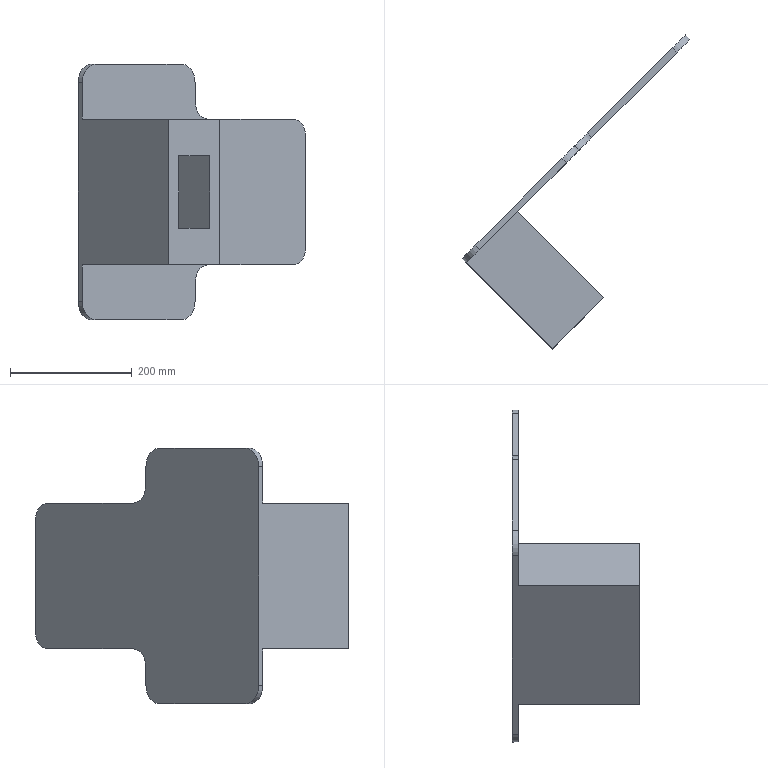Part | SolidWorks | 1 solid | 27 faces | box 374.767 x 516.188 x 420 mm | volume 5744112 mm3 | plane 19 | cylinder 8 | commonest cylinder face diameters 60 x8
STEP:
#1=CARTESIAN_POINT('',(-9.899,343.654,-1049.42));
#2=VERTEX_POINT('',#1);
#3=CARTESIAN_POINT('',(-60.811,292.742,-1049.42));
#4=VERTEX_POINT('',#3);
#5=CARTESIAN_POINT('',(-9.899,343.654,-1049.42));
#6=DIRECTION('',(-0.7071,-0.7071,0.));
#7=VECTOR('',#6,1000.);
#8=LINE('',#5,#7);
#9=EDGE_CURVE('',#2,#4,#8,.T.);
#10=ORIENTED_EDGE('',*,*,#9,.T.);
#11=CARTESIAN_POINT('',(-60.811,292.742,-1169.42));
#12=VERTEX_POINT('',#11);
#13=CARTESIAN_POINT('',(-60.811,292.742,-1169.42));
#14=DIRECTION('',(0.,0.,1.));
#15=VECTOR('',#14,1000.);
#16=LINE('',#13,#15);
#17=EDGE_CURVE('',#12,#4,#16,.T.);
#18=ORIENTED_EDGE('',*,*,#17,.F.);
#19=CARTESIAN_POINT('',(-9.899,343.654,-1169.42));
#20=VERTEX_POINT('',#19);
#21=CARTESIAN_POINT('',(-60.811,292.742,-1169.42));
#22=DIRECTION('',(0.7071,0.7071,0.));
#23=VECTOR('',#22,1000.);
#24=LINE('',#21,#23);
#25=EDGE_CURVE('',#12,#20,#24,.T.);
#26=ORIENTED_EDGE('',*,*,#25,.T.);
#27=CARTESIAN_POINT('',(-9.899,343.654,-1049.42));
#28=DIRECTION('',(0.,0.,-1.));
#29=VECTOR('',#28,1000.);
#30=LINE('',#27,#29);
#31=EDGE_CURVE('',#2,#20,#30,.T.);
#32=ORIENTED_EDGE('',*,*,#31,.F.);
#33=EDGE_LOOP('',(#10,#18,#26,#32));
#34=FACE_OUTER_BOUND('',#33,.T.);
#35=CARTESIAN_POINT('',(-77.782,275.772,-989.42));
#36=DIRECTION('',(0.7071,-0.7071,0.));
#37=DIRECTION('',(0.,0.,-1.));
#38=AXIS2_PLACEMENT_3D('',#35,#36,#37);
#39=PLANE('',#38);
#40=ADVANCED_FACE('',(#34),#39,.T.);
#41=CARTESIAN_POINT('',(131.522,202.233,-1169.42));
#42=VERTEX_POINT('',#41);
#43=CARTESIAN_POINT('',(80.61,151.321,-1169.42));
#44=VERTEX_POINT('',#43);
#45=CARTESIAN_POINT('',(131.522,202.233,-1169.42));
#46=DIRECTION('',(-0.7071,-0.7071,0.));
#47=VECTOR('',#46,1000.);
#48=LINE('',#45,#47);
#49=EDGE_CURVE('',#42,#44,#48,.T.);
#50=ORIENTED_EDGE('',*,*,#49,.F.);
#51=CARTESIAN_POINT('',(-9.899,343.654,-1169.42));
#52=DIRECTION('',(0.7071,-0.7071,0.));
#53=VECTOR('',#52,1000.);
#54=LINE('',#51,#53);
#55=EDGE_CURVE('',#20,#42,#54,.T.);
#56=ORIENTED_EDGE('',*,*,#55,.F.);
#57=ORIENTED_EDGE('',*,*,#25,.F.);
#58=CARTESIAN_POINT('',(80.61,151.321,-1169.42));
#59=DIRECTION('',(-0.7071,0.7071,0.));
#60=VECTOR('',#59,1000.);
#61=LINE('',#58,#60);
#62=EDGE_CURVE('',#44,#12,#61,.T.);
#63=ORIENTED_EDGE('',*,*,#62,.F.);
#64=EDGE_LOOP('',(#50,#56,#57,#63));
#65=FACE_OUTER_BOUND('',#64,.T.);
#66=CARTESIAN_POINT('',(80.61,151.321,-1169.42));
#67=DIRECTION('',(0.,0.,1.));
#68=DIRECTION('',(1.,0.,0.));
#69=AXIS2_PLACEMENT_3D('',#66,#67,#68);
#70=PLANE('',#69);
#71=ADVANCED_FACE('',(#65),#70,.T.);
#72=CARTESIAN_POINT('',(131.522,202.233,-1049.42));
#73=VERTEX_POINT('',#72);
#74=CARTESIAN_POINT('',(131.522,202.233,-1049.42));
#75=DIRECTION('',(0.,0.,-1.));
#76=VECTOR('',#75,1000.);
#77=LINE('',#74,#76);
#78=EDGE_CURVE('',#73,#42,#77,.T.);
#79=ORIENTED_EDGE('',*,*,#78,.F.);
#80=CARTESIAN_POINT('',(131.522,202.233,-1049.42));
#81=DIRECTION('',(-0.7071,0.7071,0.));
#82=VECTOR('',#81,1000.);
#83=LINE('',#80,#82);
#84=EDGE_CURVE('',#73,#2,#83,.T.);
#85=ORIENTED_EDGE('',*,*,#84,.T.);
#86=ORIENTED_EDGE('',*,*,#31,.T.);
#87=ORIENTED_EDGE('',*,*,#55,.T.);
#88=EDGE_LOOP('',(#79,#85,#86,#87));
#89=FACE_OUTER_BOUND('',#88,.T.);
#90=CARTESIAN_POINT('',(131.522,202.233,-1169.42));
#91=DIRECTION('',(-0.7071,-0.7071,0.));
#92=DIRECTION('',(-0.7071,0.7071,0.));
#93=AXIS2_PLACEMENT_3D('',#90,#91,#92);
#94=PLANE('',#93);
#95=ADVANCED_FACE('',(#89),#94,.T.);
#96=CARTESIAN_POINT('',(80.61,151.321,-1049.42));
#97=VERTEX_POINT('',#96);
#98=CARTESIAN_POINT('',(80.61,151.321,-1049.42));
#99=DIRECTION('',(0.7071,0.7071,0.));
#100=VECTOR('',#99,1000.);
#101=LINE('',#98,#100);
#102=EDGE_CURVE('',#97,#73,#101,.T.);
#103=ORIENTED_EDGE('',*,*,#102,.F.);
#104=CARTESIAN_POINT('',(-60.811,292.742,-1049.42));
#105=DIRECTION('',(0.7071,-0.7071,0.));
#106=VECTOR('',#105,1000.);
#107=LINE('',#104,#106);
#108=EDGE_CURVE('',#4,#97,#107,.T.);
#109=ORIENTED_EDGE('',*,*,#108,.F.);
#110=ORIENTED_EDGE('',*,*,#9,.F.);
#111=ORIENTED_EDGE('',*,*,#84,.F.);
#112=EDGE_LOOP('',(#103,#109,#110,#111));
#113=FACE_OUTER_BOUND('',#112,.T.);
#114=CARTESIAN_POINT('',(131.522,202.233,-1049.42));
#115=DIRECTION('',(0.,0.,-1.));
#116=DIRECTION('',(0.,-1.,0.));
#117=AXIS2_PLACEMENT_3D('',#114,#115,#116);
#118=PLANE('',#117);
#119=ADVANCED_FACE('',(#113),#118,.T.);
#120=CARTESIAN_POINT('',(80.61,151.321,-1169.42));
#121=DIRECTION('',(0.,0.,1.));
#122=VECTOR('',#121,1000.);
#123=LINE('',#120,#122);
#124=EDGE_CURVE('',#44,#97,#123,.T.);
#125=ORIENTED_EDGE('',*,*,#124,.F.);
#126=ORIENTED_EDGE('',*,*,#62,.T.);
#127=ORIENTED_EDGE('',*,*,#17,.T.);
#128=ORIENTED_EDGE('',*,*,#108,.T.);
#129=EDGE_LOOP('',(#125,#126,#127,#128));
#130=FACE_OUTER_BOUND('',#129,.T.);
#131=CARTESIAN_POINT('',(80.61,151.321,-1049.42));
#132=DIRECTION('',(0.7071,0.7071,0.));
#133=DIRECTION('',(0.,0.,-1.));
#134=AXIS2_PLACEMENT_3D('',#131,#132,#133);
#135=PLANE('',#134);
#136=ADVANCED_FACE('',(#130),#135,.T.);
#137=CARTESIAN_POINT('',(63.64,134.35,-989.42));
#138=VERTEX_POINT('',#137);
#139=CARTESIAN_POINT('',(-77.782,275.772,-989.42));
#140=VERTEX_POINT('',#139);
#141=CARTESIAN_POINT('',(63.64,134.35,-989.42));
#142=DIRECTION('',(-0.7071,0.7071,0.));
#143=VECTOR('',#142,1000.);
#144=LINE('',#141,#143);
#145=EDGE_CURVE('',#138,#140,#144,.T.);
#146=ORIENTED_EDGE('',*,*,#145,.F.);
#147=CARTESIAN_POINT('',(148.492,219.203,-989.42));
#148=VERTEX_POINT('',#147);
#149=CARTESIAN_POINT('',(148.492,219.203,-989.42));
#150=DIRECTION('',(-0.7071,-0.7071,0.));
#151=VECTOR('',#150,1000.);
#152=LINE('',#149,#151);
#153=EDGE_CURVE('',#148,#138,#152,.T.);
#154=ORIENTED_EDGE('',*,*,#153,.F.);
#155=CARTESIAN_POINT('',(7.071,360.624,-989.42));
#156=VERTEX_POINT('',#155);
#157=CARTESIAN_POINT('',(7.071,360.624,-989.42));
#158=DIRECTION('',(0.7071,-0.7071,0.));
#159=VECTOR('',#158,1000.);
#160=LINE('',#157,#159);
#161=EDGE_CURVE('',#156,#148,#160,.T.);
#162=ORIENTED_EDGE('',*,*,#161,.F.);
#163=CARTESIAN_POINT('',(-77.782,275.772,-989.42));
#164=DIRECTION('',(0.7071,0.7071,0.));
#165=VECTOR('',#164,1000.);
#166=LINE('',#163,#165);
#167=EDGE_CURVE('',#140,#156,#166,.T.);
#168=ORIENTED_EDGE('',*,*,#167,.F.);
#169=EDGE_LOOP('',(#146,#154,#162,#168));
#170=FACE_OUTER_BOUND('',#169,.T.);
#171=CARTESIAN_POINT('',(63.64,134.35,-989.42));
#172=DIRECTION('',(0.,0.,1.));
#173=DIRECTION('',(1.,0.,0.));
#174=AXIS2_PLACEMENT_3D('',#171,#172,#173);
#175=PLANE('',#174);
#176=ADVANCED_FACE('',(#170),#175,.T.);
#177=CARTESIAN_POINT('',(289.914,643.467,-1199.42));
#178=VERTEX_POINT('',#177);
#179=CARTESIAN_POINT('',(289.914,643.467,-1019.42));
#180=VERTEX_POINT('',#179);
#181=CARTESIAN_POINT('',(289.914,643.467,-1229.42));
#182=DIRECTION('',(0.,0.,1.));
#183=VECTOR('',#182,1000.);
#184=LINE('',#181,#183);
#185=EDGE_CURVE('',#178,#180,#184,.T.);
#186=ORIENTED_EDGE('',*,*,#185,.F.);
#187=CARTESIAN_POINT('',(282.843,650.538,-1199.42));
#188=VERTEX_POINT('',#187);
#189=CARTESIAN_POINT('',(431.335,502.046,-1199.42));
#190=DIRECTION('',(-0.7071,0.7071,0.));
#191=VECTOR('',#190,1000.);
#192=LINE('',#189,#191);
#193=EDGE_CURVE('',#178,#188,#192,.T.);
#194=ORIENTED_EDGE('',*,*,#193,.T.);
#195=CARTESIAN_POINT('',(282.843,650.538,-1019.42));
#196=VERTEX_POINT('',#195);
#197=CARTESIAN_POINT('',(282.843,650.538,-989.42));
#198=DIRECTION('',(0.,0.,-1.));
#199=VECTOR('',#198,1000.);
#200=LINE('',#197,#199);
#201=EDGE_CURVE('',#196,#188,#200,.T.);
#202=ORIENTED_EDGE('',*,*,#201,.F.);
#203=CARTESIAN_POINT('',(431.335,502.046,-1019.42));
#204=DIRECTION('',(0.7071,-0.7071,0.));
#205=VECTOR('',#204,1000.);
#206=LINE('',#203,#205);
#207=EDGE_CURVE('',#196,#180,#206,.T.);
#208=ORIENTED_EDGE('',*,*,#207,.T.);
#209=EDGE_LOOP('',(#186,#194,#202,#208));
#210=FACE_OUTER_BOUND('',#209,.T.);
#211=CARTESIAN_POINT('',(431.335,502.046,-1099.061));
#212=DIRECTION('',(0.7071,0.7071,0.));
#213=DIRECTION('',(0.,0.,-1.));
#214=AXIS2_PLACEMENT_3D('',#211,#212,#213);
#215=PLANE('',#214);
#216=ADVANCED_FACE('',(#210),#215,.T.);
#217=CARTESIAN_POINT('',(268.701,622.254,-989.42));
#218=VERTEX_POINT('',#217);
#219=CARTESIAN_POINT('',(128.787,482.34,-989.42));
#220=VERTEX_POINT('',#219);
#221=CARTESIAN_POINT('',(289.914,643.467,-989.42));
#222=DIRECTION('',(-0.7071,-0.7071,0.));
#223=VECTOR('',#222,1000.);
#224=LINE('',#221,#223);
#225=EDGE_CURVE('',#218,#220,#224,.T.);
#226=ORIENTED_EDGE('',*,*,#225,.F.);
#227=CARTESIAN_POINT('',(261.63,629.325,-989.42));
#228=VERTEX_POINT('',#227);
#229=CARTESIAN_POINT('',(410.122,480.833,-989.42));
#230=DIRECTION('',(-0.7071,0.7071,0.));
#231=VECTOR('',#230,1000.);
#232=LINE('',#229,#231);
#233=EDGE_CURVE('',#218,#228,#232,.T.);
#234=ORIENTED_EDGE('',*,*,#233,.T.);
#235=CARTESIAN_POINT('',(121.716,489.411,-989.42));
#236=VERTEX_POINT('',#235);
#237=CARTESIAN_POINT('',(100.503,468.198,-989.42));
#238=DIRECTION('',(0.7071,0.7071,0.));
#239=VECTOR('',#238,1000.);
#240=LINE('',#237,#239);
#241=EDGE_CURVE('',#236,#228,#240,.T.);
#242=ORIENTED_EDGE('',*,*,#241,.F.);
#243=CARTESIAN_POINT('',(128.787,482.34,-989.42));
#244=DIRECTION('',(0.7071,-0.7071,0.));
#245=VECTOR('',#244,1000.);
#246=LINE('',#243,#245);
#247=EDGE_CURVE('',#236,#220,#246,.T.);
#248=ORIENTED_EDGE('',*,*,#247,.T.);
#249=EDGE_LOOP('',(#226,#234,#242,#248));
#250=FACE_OUTER_BOUND('',#249,.T.);
#251=CARTESIAN_POINT('',(63.64,134.35,-989.42));
#252=DIRECTION('',(0.,0.,1.));
#253=DIRECTION('',(1.,0.,0.));
#254=AXIS2_PLACEMENT_3D('',#251,#252,#253);
#255=PLANE('',#254);
#256=ADVANCED_FACE('',(#250),#255,.T.);
#257=CARTESIAN_POINT('',(107.574,461.127,-929.42));
#258=VERTEX_POINT('',#257);
#259=CARTESIAN_POINT('',(107.574,461.127,-959.42));
#260=VERTEX_POINT('',#259);
#261=CARTESIAN_POINT('',(107.574,461.127,-899.42));
#262=DIRECTION('',(0.,0.,-1.));
#263=VECTOR('',#262,1000.);
#264=LINE('',#261,#263);
#265=EDGE_CURVE('',#258,#260,#264,.T.);
#266=ORIENTED_EDGE('',*,*,#265,.T.);
#267=CARTESIAN_POINT('',(100.503,468.198,-959.42));
#268=VERTEX_POINT('',#267);
#269=CARTESIAN_POINT('',(100.503,468.198,-959.42));
#270=DIRECTION('',(-0.7071,0.7071,0.));
#271=VECTOR('',#270,1000.);
#272=LINE('',#269,#271);
#273=EDGE_CURVE('',#260,#268,#272,.T.);
#274=ORIENTED_EDGE('',*,*,#273,.T.);
#275=CARTESIAN_POINT('',(100.503,468.198,-929.42));
#276=VERTEX_POINT('',#275);
#277=CARTESIAN_POINT('',(100.503,468.198,-899.42));
#278=DIRECTION('',(0.,0.,-1.));
#279=VECTOR('',#278,1000.);
#280=LINE('',#277,#279);
#281=EDGE_CURVE('',#276,#268,#280,.T.);
#282=ORIENTED_EDGE('',*,*,#281,.F.);
#283=CARTESIAN_POINT('',(100.503,468.198,-929.42));
#284=DIRECTION('',(0.7071,-0.7071,0.));
#285=VECTOR('',#284,1000.);
#286=LINE('',#283,#285);
#287=EDGE_CURVE('',#276,#258,#286,.T.);
#288=ORIENTED_EDGE('',*,*,#287,.T.);
#289=EDGE_LOOP('',(#266,#274,#282,#288));
#290=FACE_OUTER_BOUND('',#289,.T.);
#291=CARTESIAN_POINT('',(100.503,468.198,-899.42));
#292=DIRECTION('',(0.7071,0.7071,0.));
#293=DIRECTION('',(0.,0.,-1.));
#294=AXIS2_PLACEMENT_3D('',#291,#292,#293);
#295=PLANE('',#294);
#296=ADVANCED_FACE('',(#290),#295,.T.);
#297=CARTESIAN_POINT('',(-63.64,304.056,-899.42));
#298=VERTEX_POINT('',#297);
#299=CARTESIAN_POINT('',(79.289,446.985,-899.42));
#300=VERTEX_POINT('',#299);
#301=CARTESIAN_POINT('',(-84.853,282.843,-899.42));
#302=DIRECTION('',(0.7071,0.7071,0.));
#303=VECTOR('',#302,1000.);
#304=LINE('',#301,#303);
#305=EDGE_CURVE('',#298,#300,#304,.T.);
#306=ORIENTED_EDGE('',*,*,#305,.F.);
#307=CARTESIAN_POINT('',(-56.569,296.985,-899.42));
#308=VERTEX_POINT('',#307);
#309=CARTESIAN_POINT('',(-63.64,304.056,-899.42));
#310=DIRECTION('',(0.7071,-0.7071,0.));
#311=VECTOR('',#310,1000.);
#312=LINE('',#309,#311);
#313=EDGE_CURVE('',#298,#308,#312,.T.);
#314=ORIENTED_EDGE('',*,*,#313,.T.);
#315=CARTESIAN_POINT('',(86.36,439.914,-899.42));
#316=VERTEX_POINT('',#315);
#317=CARTESIAN_POINT('',(-77.782,275.772,-899.42));
#318=DIRECTION('',(0.7071,0.7071,0.));
#319=VECTOR('',#318,1000.);
#320=LINE('',#317,#319);
#321=EDGE_CURVE('',#308,#316,#320,.T.);
#322=ORIENTED_EDGE('',*,*,#321,.T.);
#323=CARTESIAN_POINT('',(79.289,446.985,-899.42));
#324=DIRECTION('',(-0.7071,0.7071,0.));
#325=VECTOR('',#324,1000.);
#326=LINE('',#323,#325);
#327=EDGE_CURVE('',#316,#300,#326,.T.);
#328=ORIENTED_EDGE('',*,*,#327,.T.);
#329=EDGE_LOOP('',(#306,#314,#322,#328));
#330=FACE_OUTER_BOUND('',#329,.T.);
#331=CARTESIAN_POINT('',(-84.853,282.843,-899.42));
#332=DIRECTION('',(0.,0.,1.));
#333=DIRECTION('',(0.7071,0.7071,0.));
#334=AXIS2_PLACEMENT_3D('',#331,#332,#333);
#335=PLANE('',#334);
#336=ADVANCED_FACE('',(#330),#335,.T.);
#337=CARTESIAN_POINT('',(79.289,446.985,-1319.42));
#338=VERTEX_POINT('',#337);
#339=CARTESIAN_POINT('',(-63.64,304.056,-1319.42));
#340=VERTEX_POINT('',#339);
#341=CARTESIAN_POINT('',(100.503,468.198,-1319.42));
#342=DIRECTION('',(-0.7071,-0.7071,0.));
#343=VECTOR('',#342,1000.);
#344=LINE('',#341,#343);
#345=EDGE_CURVE('',#338,#340,#344,.T.);
#346=ORIENTED_EDGE('',*,*,#345,.F.);
#347=CARTESIAN_POINT('',(86.36,439.914,-1319.42));
#348=VERTEX_POINT('',#347);
#349=CARTESIAN_POINT('',(79.289,446.985,-1319.42));
#350=DIRECTION('',(0.7071,-0.7071,0.));
#351=VECTOR('',#350,1000.);
#352=LINE('',#349,#351);
#353=EDGE_CURVE('',#338,#348,#352,.T.);
#354=ORIENTED_EDGE('',*,*,#353,.T.);
#355=CARTESIAN_POINT('',(-56.569,296.985,-1319.42));
#356=VERTEX_POINT('',#355);
#357=CARTESIAN_POINT('',(107.574,461.127,-1319.42));
#358=DIRECTION('',(-0.7071,-0.7071,0.));
#359=VECTOR('',#358,1000.);
#360=LINE('',#357,#359);
#361=EDGE_CURVE('',#348,#356,#360,.T.);
#362=ORIENTED_EDGE('',*,*,#361,.T.);
#363=CARTESIAN_POINT('',(-63.64,304.056,-1319.42));
#364=DIRECTION('',(-0.7071,0.7071,0.));
#365=VECTOR('',#364,1000.);
#366=LINE('',#363,#365);
#367=EDGE_CURVE('',#356,#340,#366,.T.);
#368=ORIENTED_EDGE('',*,*,#367,.T.);
#369=EDGE_LOOP('',(#346,#354,#362,#368));
#370=FACE_OUTER_BOUND('',#369,.T.);
#371=CARTESIAN_POINT('',(100.503,468.198,-1319.42));
#372=DIRECTION('',(0.,0.,-1.));
#373=DIRECTION('',(-0.7071,-0.7071,0.));
#374=AXIS2_PLACEMENT_3D('',#371,#372,#373);
#375=PLANE('',#374);
#376=ADVANCED_FACE('',(#370),#375,.T.);
#377=CARTESIAN_POINT('',(148.492,219.203,-1229.42));
#378=VERTEX_POINT('',#377);
#379=CARTESIAN_POINT('',(7.071,360.624,-1229.42));
#380=VERTEX_POINT('',#379);
#381=CARTESIAN_POINT('',(148.492,219.203,-1229.42));
#382=DIRECTION('',(-0.7071,0.7071,0.));
#383=VECTOR('',#382,1000.);
#384=LINE('',#381,#383);
#385=EDGE_CURVE('',#378,#380,#384,.T.);
#386=ORIENTED_EDGE('',*,*,#385,.F.);
#387=CARTESIAN_POINT('',(63.64,134.35,-1229.42));
#388=VERTEX_POINT('',#387);
#389=CARTESIAN_POINT('',(63.64,134.35,-1229.42));
#390=DIRECTION('',(0.7071,0.7071,0.));
#391=VECTOR('',#390,1000.);
#392=LINE('',#389,#391);
#393=EDGE_CURVE('',#388,#378,#392,.T.);
#394=ORIENTED_EDGE('',*,*,#393,.F.);
#395=CARTESIAN_POINT('',(-77.782,275.772,-1229.42));
#396=VERTEX_POINT('',#395);
#397=CARTESIAN_POINT('',(-77.782,275.772,-1229.42));
#398=DIRECTION('',(0.7071,-0.7071,0.));
#399=VECTOR('',#398,1000.);
#400=LINE('',#397,#399);
#401=EDGE_CURVE('',#396,#388,#400,.T.);
#402=ORIENTED_EDGE('',*,*,#401,.F.);
#403=CARTESIAN_POINT('',(7.071,360.624,-1229.42));
#404=DIRECTION('',(-0.7071,-0.7071,0.));
#405=VECTOR('',#404,1000.);
#406=LINE('',#403,#405);
#407=EDGE_CURVE('',#380,#396,#406,.T.);
#408=ORIENTED_EDGE('',*,*,#407,.F.);
#409=EDGE_LOOP('',(#386,#394,#402,#408));
#410=FACE_OUTER_BOUND('',#409,.T.);
#411=CARTESIAN_POINT('',(148.492,219.203,-1229.42));
#412=DIRECTION('',(0.,0.,-1.));
#413=DIRECTION('',(0.,-1.,0.));
#414=AXIS2_PLACEMENT_3D('',#411,#412,#413);
#415=PLANE('',#414);
#416=ADVANCED_FACE('',(#410),#415,.T.);
#417=CARTESIAN_POINT('',(-77.782,275.772,-929.42));
#418=VERTEX_POINT('',#417);
#419=CARTESIAN_POINT('',(-77.782,275.772,-989.42));
#420=DIRECTION('',(0.,0.,1.));
#421=VECTOR('',#420,1000.);
#422=LINE('',#419,#421);
#423=EDGE_CURVE('',#140,#418,#422,.T.);
#424=ORIENTED_EDGE('',*,*,#423,.T.);
#425=CARTESIAN_POINT('',(-84.853,282.843,-929.42));
#426=VERTEX_POINT('',#425);
#427=CARTESIAN_POINT('',(63.64,134.35,-929.42));
#428=DIRECTION('',(-0.7071,0.7071,0.));
#429=VECTOR('',#428,1000.);
#430=LINE('',#427,#429);
#431=EDGE_CURVE('',#418,#426,#430,.T.);
#432=ORIENTED_EDGE('',*,*,#431,.T.);
#433=CARTESIAN_POINT('',(-84.853,282.843,-1289.42));
#434=VERTEX_POINT('',#433);
#435=CARTESIAN_POINT('',(-84.853,282.843,-1319.42));
#436=DIRECTION('',(0.,0.,1.));
#437=VECTOR('',#436,1000.);
#438=LINE('',#435,#437);
#439=EDGE_CURVE('',#434,#426,#438,.T.);
#440=ORIENTED_EDGE('',*,*,#439,.F.);
#441=CARTESIAN_POINT('',(-77.782,275.772,-1289.42));
#442=VERTEX_POINT('',#441);
#443=CARTESIAN_POINT('',(63.64,134.35,-1289.42));
#444=DIRECTION('',(0.7071,-0.7071,0.));
#445=VECTOR('',#444,1000.);
#446=LINE('',#443,#445);
#447=EDGE_CURVE('',#434,#442,#446,.T.);
#448=ORIENTED_EDGE('',*,*,#447,.T.);
#449=CARTESIAN_POINT('',(-77.782,275.772,-1319.42));
#450=DIRECTION('',(0.,0.,1.));
#451=VECTOR('',#450,1000.);
#452=LINE('',#449,#451);
#453=EDGE_CURVE('',#442,#396,#452,.T.);
#454=ORIENTED_EDGE('',*,*,#453,.T.);
#455=ORIENTED_EDGE('',*,*,#401,.T.);
#456=CARTESIAN_POINT('',(63.64,134.35,-989.42));
#457=DIRECTION('',(0.,0.,-1.));
#458=VECTOR('',#457,1000.);
#459=LINE('',#456,#458);
#460=EDGE_CURVE('',#138,#388,#459,.T.);
#461=ORIENTED_EDGE('',*,*,#460,.F.);
#462=ORIENTED_EDGE('',*,*,#145,.T.);
#463=EDGE_LOOP('',(#424,#432,#440,#448,#454,#455,#461,#462));
#464=FACE_OUTER_BOUND('',#463,.T.);
#465=CARTESIAN_POINT('',(63.64,134.35,-1229.42));
#466=DIRECTION('',(-0.7071,-0.7071,0.));
#467=DIRECTION('',(-0.7071,0.7071,0.));
#468=AXIS2_PLACEMENT_3D('',#465,#466,#467);
#469=PLANE('',#468);
#470=ADVANCED_FACE('',(#464),#469,.T.);
#471=ORIENTED_EDGE('',*,*,#439,.T.);
#472=CARTESIAN_POINT('',(-63.64,304.056,-929.42));
#473=DIRECTION('',(-0.7071,0.7071,0.));
#474=DIRECTION('',(-0.7071,-0.7071,0.));
#475=AXIS2_PLACEMENT_3D('',#472,#473,#474);
#476=CIRCLE('',#475,30.);
#477=EDGE_CURVE('',#426,#298,#476,.T.);
#478=ORIENTED_EDGE('',*,*,#477,.T.);
#479=ORIENTED_EDGE('',*,*,#305,.T.);
#480=CARTESIAN_POINT('',(79.289,446.985,-929.42));
#481=DIRECTION('',(-0.7071,0.7071,0.));
#482=DIRECTION('',(-0.7071,-0.7071,0.));
#483=AXIS2_PLACEMENT_3D('',#480,#481,#482);
#484=CIRCLE('',#483,30.);
#485=EDGE_CURVE('',#300,#276,#484,.T.);
#486=ORIENTED_EDGE('',*,*,#485,.T.);
#487=ORIENTED_EDGE('',*,*,#281,.T.);
#488=CARTESIAN_POINT('',(121.716,489.411,-959.42));
#489=DIRECTION('',(0.7071,-0.7071,0.));
#490=DIRECTION('',(-0.7071,-0.7071,0.));
#491=AXIS2_PLACEMENT_3D('',#488,#489,#490);
#492=CIRCLE('',#491,30.);
#493=EDGE_CURVE('',#268,#236,#492,.T.);
#494=ORIENTED_EDGE('',*,*,#493,.T.);
#495=ORIENTED_EDGE('',*,*,#241,.T.);
#496=CARTESIAN_POINT('',(261.63,629.325,-1019.42));
#497=DIRECTION('',(-0.7071,0.7071,0.));
#498=DIRECTION('',(-0.7071,-0.7071,0.));
#499=AXIS2_PLACEMENT_3D('',#496,#497,#498);
#500=CIRCLE('',#499,30.);
#501=EDGE_CURVE('',#228,#196,#500,.T.);
#502=ORIENTED_EDGE('',*,*,#501,.T.);
#503=ORIENTED_EDGE('',*,*,#201,.T.);
#504=CARTESIAN_POINT('',(261.63,629.325,-1229.42));
#505=VERTEX_POINT('',#504);
#506=CARTESIAN_POINT('',(261.63,629.325,-1199.42));
#507=DIRECTION('',(-0.7071,0.7071,0.));
#508=DIRECTION('',(-0.7071,-0.7071,0.));
#509=AXIS2_PLACEMENT_3D('',#506,#507,#508);
#510=CIRCLE('',#509,30.);
#511=EDGE_CURVE('',#188,#505,#510,.T.);
#512=ORIENTED_EDGE('',*,*,#511,.T.);
#513=CARTESIAN_POINT('',(121.716,489.411,-1229.42));
#514=VERTEX_POINT('',#513);
#515=CARTESIAN_POINT('',(282.843,650.538,-1229.42));
#516=DIRECTION('',(-0.7071,-0.7071,0.));
#517=VECTOR('',#516,1000.);
#518=LINE('',#515,#517);
#519=EDGE_CURVE('',#505,#514,#518,.T.);
#520=ORIENTED_EDGE('',*,*,#519,.T.);
#521=CARTESIAN_POINT('',(100.503,468.198,-1259.42));
#522=VERTEX_POINT('',#521);
#523=CARTESIAN_POINT('',(121.716,489.411,-1259.42));
#524=DIRECTION('',(0.7071,-0.7071,0.));
#525=DIRECTION('',(-0.7071,-0.7071,0.));
#526=AXIS2_PLACEMENT_3D('',#523,#524,#525);
#527=CIRCLE('',#526,30.);
#528=EDGE_CURVE('',#514,#522,#527,.T.);
#529=ORIENTED_EDGE('',*,*,#528,.T.);
#530=CARTESIAN_POINT('',(100.503,468.198,-1289.42));
#531=VERTEX_POINT('',#530);
#532=CARTESIAN_POINT('',(100.503,468.198,-1229.42));
#533=DIRECTION('',(0.,0.,-1.));
#534=VECTOR('',#533,1000.);
#535=LINE('',#532,#534);
#536=EDGE_CURVE('',#522,#531,#535,.T.);
#537=ORIENTED_EDGE('',*,*,#536,.T.);
#538=CARTESIAN_POINT('',(79.289,446.985,-1289.42));
#539=DIRECTION('',(-0.7071,0.7071,0.));
#540=DIRECTION('',(-0.7071,-0.7071,0.));
#541=AXIS2_PLACEMENT_3D('',#538,#539,#540);
#542=CIRCLE('',#541,30.);
#543=EDGE_CURVE('',#531,#338,#542,.T.);
#544=ORIENTED_EDGE('',*,*,#543,.T.);
#545=ORIENTED_EDGE('',*,*,#345,.T.);
#546=CARTESIAN_POINT('',(-63.64,304.056,-1289.42));
#547=DIRECTION('',(-0.7071,0.7071,0.));
#548=DIRECTION('',(-0.7071,-0.7071,0.));
#549=AXIS2_PLACEMENT_3D('',#546,#547,#548);
#550=CIRCLE('',#549,30.);
#551=EDGE_CURVE('',#340,#434,#550,.T.);
#552=ORIENTED_EDGE('',*,*,#551,.T.);
#553=EDGE_LOOP('',(#471,#478,#479,#486,#487,#494,#495,#502,#503,#512,#520,#529,#537,#544,#545,#552));
#554=FACE_OUTER_BOUND('',#553,.T.);
#555=CARTESIAN_POINT('',(-84.853,282.843,-1099.061));
#556=DIRECTION('',(-0.7071,0.7071,0.));
#557=DIRECTION('',(0.,0.,1.));
#558=AXIS2_PLACEMENT_3D('',#555,#556,#557);
#559=PLANE('',#558);
#560=ADVANCED_FACE('',(#554),#559,.T.);
#561=CARTESIAN_POINT('',(107.574,461.127,-1259.42));
#562=VERTEX_POINT('',#561);
#563=CARTESIAN_POINT('',(107.574,461.127,-1289.42));
#564=VERTEX_POINT('',#563);
#565=CARTESIAN_POINT('',(107.574,461.127,-1229.42));
#566=DIRECTION('',(0.,0.,-1.));
#567=VECTOR('',#566,1000.);
#568=LINE('',#565,#567);
#569=EDGE_CURVE('',#562,#564,#568,.T.);
#570=ORIENTED_EDGE('',*,*,#569,.T.);
#571=CARTESIAN_POINT('',(100.503,468.198,-1289.42));
#572=DIRECTION('',(-0.7071,0.7071,0.));
#573=VECTOR('',#572,1000.);
#574=LINE('',#571,#573);
#575=EDGE_CURVE('',#564,#531,#574,.T.);
#576=ORIENTED_EDGE('',*,*,#575,.T.);
#577=ORIENTED_EDGE('',*,*,#536,.F.);
#578=CARTESIAN_POINT('',(107.574,461.127,-1259.42));
#579=DIRECTION('',(0.7071,-0.7071,0.));
#580=VECTOR('',#579,1000.);
#581=LINE('',#578,#580);
#582=EDGE_CURVE('',#522,#562,#581,.T.);
#583=ORIENTED_EDGE('',*,*,#582,.T.);
#584=EDGE_LOOP('',(#570,#576,#577,#583));
#585=FACE_OUTER_BOUND('',#584,.T.);
#586=CARTESIAN_POINT('',(100.503,468.198,-1229.42));
#587=DIRECTION('',(0.7071,0.7071,0.));
#588=DIRECTION('',(0.,0.,-1.));
#589=AXIS2_PLACEMENT_3D('',#586,#587,#588);
#590=PLANE('',#589);
#591=ADVANCED_FACE('',(#585),#590,.T.);
#592=CARTESIAN_POINT('',(128.787,482.34,-1229.42));
#593=VERTEX_POINT('',#592);
#594=CARTESIAN_POINT('',(268.701,622.254,-1229.42));
#595=VERTEX_POINT('',#594);
#596=CARTESIAN_POINT('',(107.574,461.127,-1229.42));
#597=DIRECTION('',(0.7071,0.7071,0.));
#598=VECTOR('',#597,1000.);
#599=LINE('',#596,#598);
#600=EDGE_CURVE('',#593,#595,#599,.T.);
#601=ORIENTED_EDGE('',*,*,#600,.F.);
#602=CARTESIAN_POINT('',(121.716,489.411,-1229.42));
#603=DIRECTION('',(-0.7071,0.7071,0.));
#604=VECTOR('',#603,1000.);
#605=LINE('',#602,#604);
#606=EDGE_CURVE('',#593,#514,#605,.T.);
#607=ORIENTED_EDGE('',*,*,#606,.T.);
#608=ORIENTED_EDGE('',*,*,#519,.F.);
#609=CARTESIAN_POINT('',(410.122,480.833,-1229.42));
#610=DIRECTION('',(0.7071,-0.7071,0.));
#611=VECTOR('',#610,1000.);
#612=LINE('',#609,#611);
#613=EDGE_CURVE('',#505,#595,#612,.T.);
#614=ORIENTED_EDGE('',*,*,#613,.T.);
#615=EDGE_LOOP('',(#601,#607,#608,#614));
#616=FACE_OUTER_BOUND('',#615,.T.);
#617=CARTESIAN_POINT('',(148.492,219.203,-1229.42));
#618=DIRECTION('',(0.,0.,-1.));
#619=DIRECTION('',(0.,-1.,0.));
#620=AXIS2_PLACEMENT_3D('',#617,#618,#619);
#621=PLANE('',#620);
#622=ADVANCED_FACE('',(#616),#621,.T.);
#623=ORIENTED_EDGE('',*,*,#321,.F.);
#624=CARTESIAN_POINT('',(-56.569,296.985,-929.42));
#625=DIRECTION('',(0.7071,-0.7071,0.));
#626=DIRECTION('',(0.7071,0.7071,0.));
#627=AXIS2_PLACEMENT_3D('',#624,#625,#626);
#628=CIRCLE('',#627,30.);
#629=EDGE_CURVE('',#308,#418,#628,.T.);
#630=ORIENTED_EDGE('',*,*,#629,.T.);
#631=ORIENTED_EDGE('',*,*,#423,.F.);
#632=ORIENTED_EDGE('',*,*,#167,.T.);
#633=CARTESIAN_POINT('',(7.071,360.624,-1229.42));
#634=DIRECTION('',(0.,0.,1.));
#635=VECTOR('',#634,1000.);
#636=LINE('',#633,#635);
#637=EDGE_CURVE('',#380,#156,#636,.T.);
#638=ORIENTED_EDGE('',*,*,#637,.F.);
#639=ORIENTED_EDGE('',*,*,#407,.T.);
#640=ORIENTED_EDGE('',*,*,#453,.F.);
#641=CARTESIAN_POINT('',(-56.569,296.985,-1289.42));
#642=DIRECTION('',(0.7071,-0.7071,0.));
#643=DIRECTION('',(0.7071,0.7071,0.));
#644=AXIS2_PLACEMENT_3D('',#641,#642,#643);
#645=CIRCLE('',#644,30.);
#646=EDGE_CURVE('',#442,#356,#645,.T.);
#647=ORIENTED_EDGE('',*,*,#646,.T.);
#648=ORIENTED_EDGE('',*,*,#361,.F.);
#649=CARTESIAN_POINT('',(86.36,439.914,-1289.42));
#650=DIRECTION('',(0.7071,-0.7071,0.));
#651=DIRECTION('',(0.7071,0.7071,0.));
#652=AXIS2_PLACEMENT_3D('',#649,#650,#651);
#653=CIRCLE('',#652,30.);
#654=EDGE_CURVE('',#348,#564,#653,.T.);
#655=ORIENTED_EDGE('',*,*,#654,.T.);
#656=ORIENTED_EDGE('',*,*,#569,.F.);
#657=CARTESIAN_POINT('',(128.787,482.34,-1259.42));
#658=DIRECTION('',(-0.7071,0.7071,0.));
#659=DIRECTION('',(0.7071,0.7071,0.));
#660=AXIS2_PLACEMENT_3D('',#657,#658,#659);
#661=CIRCLE('',#660,30.);
#662=EDGE_CURVE('',#562,#593,#661,.T.);
#663=ORIENTED_EDGE('',*,*,#662,.T.);
#664=ORIENTED_EDGE('',*,*,#600,.T.);
#665=CARTESIAN_POINT('',(268.701,622.254,-1199.42));
#666=DIRECTION('',(0.7071,-0.7071,0.));
#667=DIRECTION('',(0.7071,0.7071,0.));
#668=AXIS2_PLACEMENT_3D('',#665,#666,#667);
#669=CIRCLE('',#668,30.);
#670=EDGE_CURVE('',#595,#178,#669,.T.);
#671=ORIENTED_EDGE('',*,*,#670,.T.);
#672=ORIENTED_EDGE('',*,*,#185,.T.);
#673=CARTESIAN_POINT('',(268.701,622.254,-1019.42));
#674=DIRECTION('',(0.7071,-0.7071,0.));
#675=DIRECTION('',(0.7071,0.7071,0.));
#676=AXIS2_PLACEMENT_3D('',#673,#674,#675);
#677=CIRCLE('',#676,30.);
#678=EDGE_CURVE('',#180,#218,#677,.T.);
#679=ORIENTED_EDGE('',*,*,#678,.T.);
#680=ORIENTED_EDGE('',*,*,#225,.T.);
#681=CARTESIAN_POINT('',(128.787,482.34,-959.42));
#682=DIRECTION('',(-0.7071,0.7071,0.));
#683=DIRECTION('',(0.7071,0.7071,0.));
#684=AXIS2_PLACEMENT_3D('',#681,#682,#683);
#685=CIRCLE('',#684,30.);
#686=EDGE_CURVE('',#220,#260,#685,.T.);
#687=ORIENTED_EDGE('',*,*,#686,.T.);
#688=ORIENTED_EDGE('',*,*,#265,.F.);
#689=CARTESIAN_POINT('',(86.36,439.914,-929.42));
#690=DIRECTION('',(0.7071,-0.7071,0.));
#691=DIRECTION('',(0.7071,0.7071,0.));
#692=AXIS2_PLACEMENT_3D('',#689,#690,#691);
#693=CIRCLE('',#692,30.);
#694=EDGE_CURVE('',#258,#316,#693,.T.);
#695=ORIENTED_EDGE('',*,*,#694,.T.);
#696=EDGE_LOOP('',(#623,#630,#631,#632,#638,#639,#640,#647,#648,#655,#656,#663,#664,#671,#672,#679,#680,#687,#688,#695));
#697=FACE_OUTER_BOUND('',#696,.T.);
#698=CARTESIAN_POINT('',(-77.782,275.772,-989.42));
#699=DIRECTION('',(0.7071,-0.7071,0.));
#700=DIRECTION('',(0.,0.,-1.));
#701=AXIS2_PLACEMENT_3D('',#698,#699,#700);
#702=PLANE('',#701);
#703=ADVANCED_FACE('',(#697),#702,.T.);
#704=ORIENTED_EDGE('',*,*,#161,.T.);
#705=CARTESIAN_POINT('',(148.492,219.203,-1229.42));
#706=DIRECTION('',(0.,0.,1.));
#707=VECTOR('',#706,1000.);
#708=LINE('',#705,#707);
#709=EDGE_CURVE('',#378,#148,#708,.T.);
#710=ORIENTED_EDGE('',*,*,#709,.F.);
#711=ORIENTED_EDGE('',*,*,#385,.T.);
#712=ORIENTED_EDGE('',*,*,#637,.T.);
#713=EDGE_LOOP('',(#704,#710,#711,#712));
#714=FACE_OUTER_BOUND('',#713,.T.);
#715=CARTESIAN_POINT('',(148.492,219.203,-989.42));
#716=DIRECTION('',(0.7071,0.7071,0.));
#717=DIRECTION('',(0.,0.,-1.));
#718=AXIS2_PLACEMENT_3D('',#715,#716,#717);
#719=PLANE('',#718);
#720=ADVANCED_FACE('',(#714),#719,.T.);
#721=ORIENTED_EDGE('',*,*,#102,.T.);
#722=ORIENTED_EDGE('',*,*,#78,.T.);
#723=ORIENTED_EDGE('',*,*,#49,.T.);
#724=ORIENTED_EDGE('',*,*,#124,.T.);
#725=EDGE_LOOP('',(#721,#722,#723,#724));
#726=FACE_BOUND('',#725,.T.);
#727=ORIENTED_EDGE('',*,*,#153,.T.);
#728=ORIENTED_EDGE('',*,*,#460,.T.);
#729=ORIENTED_EDGE('',*,*,#393,.T.);
#730=ORIENTED_EDGE('',*,*,#709,.T.);
#731=EDGE_LOOP('',(#727,#728,#729,#730));
#732=FACE_OUTER_BOUND('',#731,.T.);
#733=CARTESIAN_POINT('',(63.64,134.35,-1099.061));
#734=DIRECTION('',(-0.7071,0.7071,0.));
#735=DIRECTION('',(0.,0.,1.));
#736=AXIS2_PLACEMENT_3D('',#733,#734,#735);
#737=PLANE('',#736);
#738=ADVANCED_FACE('',(#726,#732),#737,.F.);
#739=ORIENTED_EDGE('',*,*,#477,.F.);
#740=ORIENTED_EDGE('',*,*,#431,.F.);
#741=ORIENTED_EDGE('',*,*,#629,.F.);
#742=ORIENTED_EDGE('',*,*,#313,.F.);
#743=EDGE_LOOP('',(#739,#740,#741,#742));
#744=FACE_OUTER_BOUND('',#743,.T.);
#745=CARTESIAN_POINT('',(-63.64,304.056,-929.42));
#746=DIRECTION('',(0.7071,-0.7071,0.));
#747=DIRECTION('',(0.7071,0.7071,0.));
#748=AXIS2_PLACEMENT_3D('',#745,#746,#747);
#749=CYLINDRICAL_SURFACE('',#748,30.);
#750=ADVANCED_FACE('',(#744),#749,.T.);
#751=ORIENTED_EDGE('',*,*,#543,.F.);
#752=ORIENTED_EDGE('',*,*,#575,.F.);
#753=ORIENTED_EDGE('',*,*,#654,.F.);
#754=ORIENTED_EDGE('',*,*,#353,.F.);
#755=EDGE_LOOP('',(#751,#752,#753,#754));
#756=FACE_OUTER_BOUND('',#755,.T.);
#757=CARTESIAN_POINT('',(79.289,446.985,-1289.42));
#758=DIRECTION('',(0.7071,-0.7071,0.));
#759=DIRECTION('',(0.7071,0.7071,0.));
#760=AXIS2_PLACEMENT_3D('',#757,#758,#759);
#761=CYLINDRICAL_SURFACE('',#760,30.);
#762=ADVANCED_FACE('',(#756),#761,.T.);
#763=ORIENTED_EDGE('',*,*,#528,.F.);
#764=ORIENTED_EDGE('',*,*,#606,.F.);
#765=ORIENTED_EDGE('',*,*,#662,.F.);
#766=ORIENTED_EDGE('',*,*,#582,.F.);
#767=EDGE_LOOP('',(#763,#764,#765,#766));
#768=FACE_OUTER_BOUND('',#767,.T.);
#769=CARTESIAN_POINT('',(121.716,489.411,-1259.42));
#770=DIRECTION('',(-0.7071,0.7071,0.));
#771=DIRECTION('',(-0.7071,-0.7071,0.));
#772=AXIS2_PLACEMENT_3D('',#769,#770,#771);
#773=CYLINDRICAL_SURFACE('',#772,30.);
#774=ADVANCED_FACE('',(#768),#773,.F.);
#775=ORIENTED_EDGE('',*,*,#670,.F.);
#776=ORIENTED_EDGE('',*,*,#613,.F.);
#777=ORIENTED_EDGE('',*,*,#511,.F.);
#778=ORIENTED_EDGE('',*,*,#193,.F.);
#779=EDGE_LOOP('',(#775,#776,#777,#778));
#780=FACE_OUTER_BOUND('',#779,.T.);
#781=CARTESIAN_POINT('',(410.122,480.833,-1199.42));
#782=DIRECTION('',(-0.7071,0.7071,0.));
#783=DIRECTION('',(-0.7071,-0.7071,0.));
#784=AXIS2_PLACEMENT_3D('',#781,#782,#783);
#785=CYLINDRICAL_SURFACE('',#784,30.);
#786=ADVANCED_FACE('',(#780),#785,.T.);
#787=ORIENTED_EDGE('',*,*,#501,.F.);
#788=ORIENTED_EDGE('',*,*,#233,.F.);
#789=ORIENTED_EDGE('',*,*,#678,.F.);
#790=ORIENTED_EDGE('',*,*,#207,.F.);
#791=EDGE_LOOP('',(#787,#788,#789,#790));
#792=FACE_OUTER_BOUND('',#791,.T.);
#793=CARTESIAN_POINT('',(410.122,480.833,-1019.42));
#794=DIRECTION('',(0.7071,-0.7071,0.));
#795=DIRECTION('',(0.7071,0.7071,0.));
#796=AXIS2_PLACEMENT_3D('',#793,#794,#795);
#797=CYLINDRICAL_SURFACE('',#796,30.);
#798=ADVANCED_FACE('',(#792),#797,.T.);
#799=ORIENTED_EDGE('',*,*,#686,.F.);
#800=ORIENTED_EDGE('',*,*,#247,.F.);
#801=ORIENTED_EDGE('',*,*,#493,.F.);
#802=ORIENTED_EDGE('',*,*,#273,.F.);
#803=EDGE_LOOP('',(#799,#800,#801,#802));
#804=FACE_OUTER_BOUND('',#803,.T.);
#805=CARTESIAN_POINT('',(121.716,489.411,-959.42));
#806=DIRECTION('',(0.7071,-0.7071,0.));
#807=DIRECTION('',(0.7071,0.7071,0.));
#808=AXIS2_PLACEMENT_3D('',#805,#806,#807);
#809=CYLINDRICAL_SURFACE('',#808,30.);
#810=ADVANCED_FACE('',(#804),#809,.F.);
#811=ORIENTED_EDGE('',*,*,#485,.F.);
#812=ORIENTED_EDGE('',*,*,#327,.F.);
#813=ORIENTED_EDGE('',*,*,#694,.F.);
#814=ORIENTED_EDGE('',*,*,#287,.F.);
#815=EDGE_LOOP('',(#811,#812,#813,#814));
#816=FACE_OUTER_BOUND('',#815,.T.);
#817=CARTESIAN_POINT('',(79.289,446.985,-929.42));
#818=DIRECTION('',(0.7071,-0.7071,0.));
#819=DIRECTION('',(0.7071,0.7071,0.));
#820=AXIS2_PLACEMENT_3D('',#817,#818,#819);
#821=CYLINDRICAL_SURFACE('',#820,30.);
#822=ADVANCED_FACE('',(#816),#821,.T.);
#823=ORIENTED_EDGE('',*,*,#551,.F.);
#824=ORIENTED_EDGE('',*,*,#367,.F.);
#825=ORIENTED_EDGE('',*,*,#646,.F.);
#826=ORIENTED_EDGE('',*,*,#447,.F.);
#827=EDGE_LOOP('',(#823,#824,#825,#826));
#828=FACE_OUTER_BOUND('',#827,.T.);
#829=CARTESIAN_POINT('',(84.853,155.563,-1289.42));
#830=DIRECTION('',(0.7071,-0.7071,0.));
#831=DIRECTION('',(0.7071,0.7071,0.));
#832=AXIS2_PLACEMENT_3D('',#829,#830,#831);
#833=CYLINDRICAL_SURFACE('',#832,30.);
#834=ADVANCED_FACE('',(#828),#833,.T.);
#835=CLOSED_SHELL('',(#40,#71,#95,#119,#136,#176,#216,#256,#296,#336,#376,#416,#470,#560,#591,#622,#703,#720,#738,#750,#762,#774,#786,#798,#810,#822,#834));
#836=MANIFOLD_SOLID_BREP('',#835);
#837=CARTESIAN_POINT('',(0.,0.,0.));
#838=DIRECTION('',(0.,0.,1.));
#839=DIRECTION('',(1.,0.,0.));
#840=AXIS2_PLACEMENT_3D('',#837,#838,#839);
#841=(LENGTH_UNIT()NAMED_UNIT(*)SI_UNIT(.MILLI.,.METRE.));
#842=UNCERTAINTY_MEASURE_WITH_UNIT(LENGTH_MEASURE(0.00001),#841,'','');
#843=(NAMED_UNIT(*)PLANE_ANGLE_UNIT()SI_UNIT($,.RADIAN.));
#844=(NAMED_UNIT(*)SI_UNIT($,.STERADIAN.)SOLID_ANGLE_UNIT());
#845=(GEOMETRIC_REPRESENTATION_CONTEXT(3)GLOBAL_UNCERTAINTY_ASSIGNED_CONTEXT((#842))GLOBAL_UNIT_ASSIGNED_CONTEXT((#841,#843,#844))REPRESENTATION_CONTEXT('',''));
#846=ADVANCED_BREP_SHAPE_REPRESENTATION('',(#836,#840),#845);